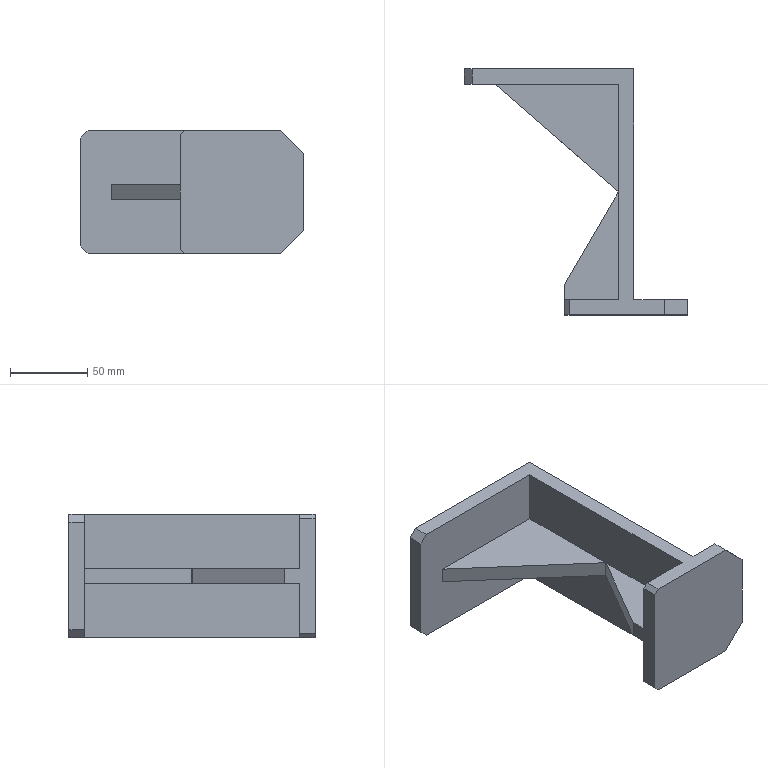Part | STEP file | Hook plate | 1 solid | 25 faces | box 145 x 159.75 x 80 mm | volume 303088 mm3 | plane 25